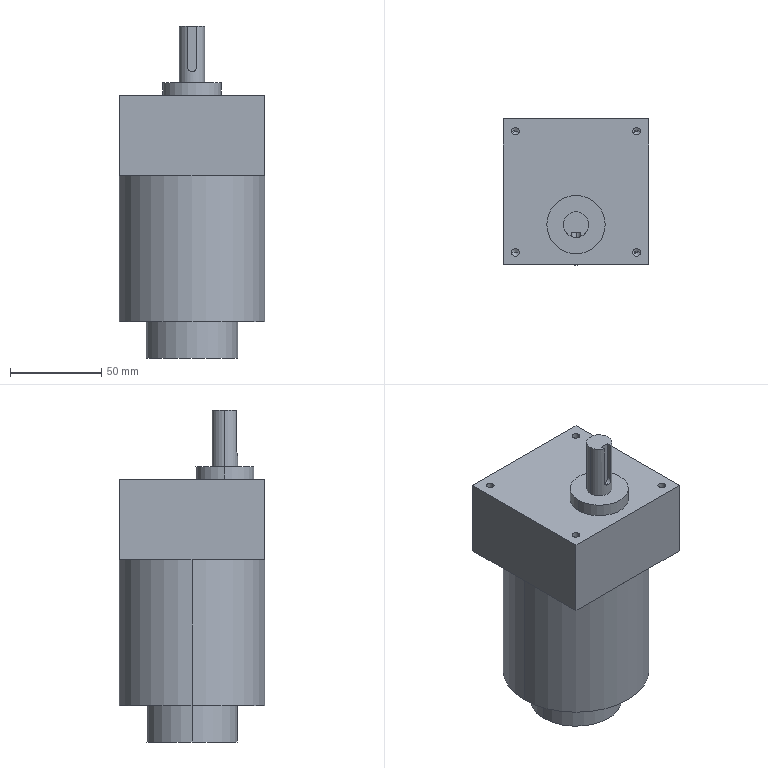Part | STEP file | Cut-off geared motor | 1 solid | 42 faces | box 80 x 80 x 182 mm | volume 732361 mm3 | cylinder 18 | plane 16 | cone 8 | commonest cylinder face diameters 4.2 x8 5 x2 14 x2 32 x2 50 x2 80 x2
STEP:
#1=CARTESIAN_POINT('',(31.134,-33.234,31.6));
#2=VERTEX_POINT('',#1);
#3=CARTESIAN_POINT('',(35.334,-33.234,31.6));
#4=VERTEX_POINT('',#3);
#5=CARTESIAN_POINT('',(33.234,-33.234,31.6));
#6=DIRECTION('',(0.,0.,1.));
#7=DIRECTION('',(1.,0.,0.));
#8=AXIS2_PLACEMENT_3D('',#5,#6,#7);
#9=CIRCLE('',#8,2.1);
#10=EDGE_CURVE('',#2,#4,#9,.T.);
#11=ORIENTED_EDGE('',*,*,#10,.F.);
#12=CARTESIAN_POINT('',(31.134,-33.234,44.));
#13=VERTEX_POINT('',#12);
#14=CARTESIAN_POINT('',(31.134,-33.234,44.));
#15=DIRECTION('',(0.,0.,1.));
#16=VECTOR('',#15,1000.);
#17=LINE('',#14,#16);
#18=EDGE_CURVE('',#2,#13,#17,.T.);
#19=ORIENTED_EDGE('',*,*,#18,.T.);
#20=CARTESIAN_POINT('',(35.334,-33.234,44.));
#21=VERTEX_POINT('',#20);
#22=CARTESIAN_POINT('',(33.234,-33.234,44.));
#23=DIRECTION('',(0.,0.,1.));
#24=DIRECTION('',(1.,0.,0.));
#25=AXIS2_PLACEMENT_3D('',#22,#23,#24);
#26=CIRCLE('',#25,2.1);
#27=EDGE_CURVE('',#13,#21,#26,.T.);
#28=ORIENTED_EDGE('',*,*,#27,.T.);
#29=CARTESIAN_POINT('',(35.334,-33.234,44.));
#30=DIRECTION('',(0.,0.,1.));
#31=VECTOR('',#30,1000.);
#32=LINE('',#29,#31);
#33=EDGE_CURVE('',#4,#21,#32,.T.);
#34=ORIENTED_EDGE('',*,*,#33,.F.);
#35=EDGE_LOOP('',(#11,#19,#28,#34));
#36=FACE_OUTER_BOUND('',#35,.T.);
#37=CARTESIAN_POINT('',(33.234,-33.234,44.));
#38=DIRECTION('',(0.,0.,1.));
#39=DIRECTION('',(1.,0.,0.));
#40=AXIS2_PLACEMENT_3D('',#37,#38,#39);
#41=CYLINDRICAL_SURFACE('',#40,2.1);
#42=ADVANCED_FACE('',(#36),#41,.F.);
#43=CARTESIAN_POINT('',(33.234,-33.234,30.338));
#44=VERTEX_POINT('',#43);
#45=CARTESIAN_POINT('',(35.334,-33.234,31.6));
#46=DIRECTION('',(0.8572,0.,0.515));
#47=VECTOR('',#46,1000.);
#48=LINE('',#45,#47);
#49=EDGE_CURVE('',#44,#4,#48,.T.);
#50=ORIENTED_EDGE('',*,*,#49,.F.);
#51=CARTESIAN_POINT('',(31.134,-33.234,31.6));
#52=DIRECTION('',(-0.8572,0.,0.515));
#53=VECTOR('',#52,1000.);
#54=LINE('',#51,#53);
#55=EDGE_CURVE('',#44,#2,#54,.T.);
#56=ORIENTED_EDGE('',*,*,#55,.T.);
#57=ORIENTED_EDGE('',*,*,#10,.T.);
#58=EDGE_LOOP('',(#50,#56,#57));
#59=FACE_OUTER_BOUND('',#58,.T.);
#60=CARTESIAN_POINT('',(33.234,-33.234,31.6));
#61=DIRECTION('',(0.,0.,1.));
#62=DIRECTION('',(1.,0.,0.));
#63=AXIS2_PLACEMENT_3D('',#60,#61,#62);
#64=CONICAL_SURFACE('',#63,2.1,1.03);
#65=ADVANCED_FACE('',(#59),#64,.F.);
#66=CARTESIAN_POINT('',(-35.334,-33.234,31.6));
#67=VERTEX_POINT('',#66);
#68=CARTESIAN_POINT('',(-31.134,-33.234,31.6));
#69=VERTEX_POINT('',#68);
#70=CARTESIAN_POINT('',(-33.234,-33.234,31.6));
#71=DIRECTION('',(0.,0.,1.));
#72=DIRECTION('',(1.,0.,0.));
#73=AXIS2_PLACEMENT_3D('',#70,#71,#72);
#74=CIRCLE('',#73,2.1);
#75=EDGE_CURVE('',#67,#69,#74,.T.);
#76=ORIENTED_EDGE('',*,*,#75,.F.);
#77=CARTESIAN_POINT('',(-35.334,-33.234,44.));
#78=VERTEX_POINT('',#77);
#79=CARTESIAN_POINT('',(-35.334,-33.234,44.));
#80=DIRECTION('',(0.,0.,1.));
#81=VECTOR('',#80,1000.);
#82=LINE('',#79,#81);
#83=EDGE_CURVE('',#67,#78,#82,.T.);
#84=ORIENTED_EDGE('',*,*,#83,.T.);
#85=CARTESIAN_POINT('',(-31.134,-33.234,44.));
#86=VERTEX_POINT('',#85);
#87=CARTESIAN_POINT('',(-33.234,-33.234,44.));
#88=DIRECTION('',(0.,0.,1.));
#89=DIRECTION('',(1.,0.,0.));
#90=AXIS2_PLACEMENT_3D('',#87,#88,#89);
#91=CIRCLE('',#90,2.1);
#92=EDGE_CURVE('',#78,#86,#91,.T.);
#93=ORIENTED_EDGE('',*,*,#92,.T.);
#94=CARTESIAN_POINT('',(-31.134,-33.234,44.));
#95=DIRECTION('',(0.,0.,1.));
#96=VECTOR('',#95,1000.);
#97=LINE('',#94,#96);
#98=EDGE_CURVE('',#69,#86,#97,.T.);
#99=ORIENTED_EDGE('',*,*,#98,.F.);
#100=EDGE_LOOP('',(#76,#84,#93,#99));
#101=FACE_OUTER_BOUND('',#100,.T.);
#102=CARTESIAN_POINT('',(-33.234,-33.234,44.));
#103=DIRECTION('',(0.,0.,1.));
#104=DIRECTION('',(1.,0.,0.));
#105=AXIS2_PLACEMENT_3D('',#102,#103,#104);
#106=CYLINDRICAL_SURFACE('',#105,2.1);
#107=ADVANCED_FACE('',(#101),#106,.F.);
#108=CARTESIAN_POINT('',(-33.234,-33.234,30.338));
#109=VERTEX_POINT('',#108);
#110=CARTESIAN_POINT('',(-31.134,-33.234,31.6));
#111=DIRECTION('',(0.8572,0.,0.515));
#112=VECTOR('',#111,1000.);
#113=LINE('',#110,#112);
#114=EDGE_CURVE('',#109,#69,#113,.T.);
#115=ORIENTED_EDGE('',*,*,#114,.F.);
#116=CARTESIAN_POINT('',(-35.334,-33.234,31.6));
#117=DIRECTION('',(-0.8572,0.,0.515));
#118=VECTOR('',#117,1000.);
#119=LINE('',#116,#118);
#120=EDGE_CURVE('',#109,#67,#119,.T.);
#121=ORIENTED_EDGE('',*,*,#120,.T.);
#122=ORIENTED_EDGE('',*,*,#75,.T.);
#123=EDGE_LOOP('',(#115,#121,#122));
#124=FACE_OUTER_BOUND('',#123,.T.);
#125=CARTESIAN_POINT('',(-33.234,-33.234,31.6));
#126=DIRECTION('',(0.,0.,1.));
#127=DIRECTION('',(1.,0.,0.));
#128=AXIS2_PLACEMENT_3D('',#125,#126,#127);
#129=CONICAL_SURFACE('',#128,2.1,1.03);
#130=ADVANCED_FACE('',(#124),#129,.F.);
#131=CARTESIAN_POINT('',(-35.334,33.234,31.6));
#132=VERTEX_POINT('',#131);
#133=CARTESIAN_POINT('',(-31.134,33.234,31.6));
#134=VERTEX_POINT('',#133);
#135=CARTESIAN_POINT('',(-33.234,33.234,31.6));
#136=DIRECTION('',(0.,0.,1.));
#137=DIRECTION('',(1.,0.,0.));
#138=AXIS2_PLACEMENT_3D('',#135,#136,#137);
#139=CIRCLE('',#138,2.1);
#140=EDGE_CURVE('',#132,#134,#139,.T.);
#141=ORIENTED_EDGE('',*,*,#140,.F.);
#142=CARTESIAN_POINT('',(-35.334,33.234,44.));
#143=VERTEX_POINT('',#142);
#144=CARTESIAN_POINT('',(-35.334,33.234,44.));
#145=DIRECTION('',(0.,0.,1.));
#146=VECTOR('',#145,1000.);
#147=LINE('',#144,#146);
#148=EDGE_CURVE('',#132,#143,#147,.T.);
#149=ORIENTED_EDGE('',*,*,#148,.T.);
#150=CARTESIAN_POINT('',(-31.134,33.234,44.));
#151=VERTEX_POINT('',#150);
#152=CARTESIAN_POINT('',(-33.234,33.234,44.));
#153=DIRECTION('',(0.,0.,1.));
#154=DIRECTION('',(1.,0.,0.));
#155=AXIS2_PLACEMENT_3D('',#152,#153,#154);
#156=CIRCLE('',#155,2.1);
#157=EDGE_CURVE('',#143,#151,#156,.T.);
#158=ORIENTED_EDGE('',*,*,#157,.T.);
#159=CARTESIAN_POINT('',(-31.134,33.234,44.));
#160=DIRECTION('',(0.,0.,1.));
#161=VECTOR('',#160,1000.);
#162=LINE('',#159,#161);
#163=EDGE_CURVE('',#134,#151,#162,.T.);
#164=ORIENTED_EDGE('',*,*,#163,.F.);
#165=EDGE_LOOP('',(#141,#149,#158,#164));
#166=FACE_OUTER_BOUND('',#165,.T.);
#167=CARTESIAN_POINT('',(-33.234,33.234,44.));
#168=DIRECTION('',(0.,0.,1.));
#169=DIRECTION('',(1.,0.,0.));
#170=AXIS2_PLACEMENT_3D('',#167,#168,#169);
#171=CYLINDRICAL_SURFACE('',#170,2.1);
#172=ADVANCED_FACE('',(#166),#171,.F.);
#173=CARTESIAN_POINT('',(-33.234,33.234,30.338));
#174=VERTEX_POINT('',#173);
#175=CARTESIAN_POINT('',(-31.134,33.234,31.6));
#176=DIRECTION('',(0.8572,0.,0.515));
#177=VECTOR('',#176,1000.);
#178=LINE('',#175,#177);
#179=EDGE_CURVE('',#174,#134,#178,.T.);
#180=ORIENTED_EDGE('',*,*,#179,.F.);
#181=CARTESIAN_POINT('',(-35.334,33.234,31.6));
#182=DIRECTION('',(-0.8572,0.,0.515));
#183=VECTOR('',#182,1000.);
#184=LINE('',#181,#183);
#185=EDGE_CURVE('',#174,#132,#184,.T.);
#186=ORIENTED_EDGE('',*,*,#185,.T.);
#187=ORIENTED_EDGE('',*,*,#140,.T.);
#188=EDGE_LOOP('',(#180,#186,#187));
#189=FACE_OUTER_BOUND('',#188,.T.);
#190=CARTESIAN_POINT('',(-33.234,33.234,31.6));
#191=DIRECTION('',(0.,0.,1.));
#192=DIRECTION('',(1.,0.,0.));
#193=AXIS2_PLACEMENT_3D('',#190,#191,#192);
#194=CONICAL_SURFACE('',#193,2.1,1.03);
#195=ADVANCED_FACE('',(#189),#194,.F.);
#196=CARTESIAN_POINT('',(31.134,33.234,31.6));
#197=VERTEX_POINT('',#196);
#198=CARTESIAN_POINT('',(35.334,33.234,31.6));
#199=VERTEX_POINT('',#198);
#200=CARTESIAN_POINT('',(33.234,33.234,31.6));
#201=DIRECTION('',(0.,0.,1.));
#202=DIRECTION('',(1.,0.,0.));
#203=AXIS2_PLACEMENT_3D('',#200,#201,#202);
#204=CIRCLE('',#203,2.1);
#205=EDGE_CURVE('',#197,#199,#204,.T.);
#206=ORIENTED_EDGE('',*,*,#205,.F.);
#207=CARTESIAN_POINT('',(31.134,33.234,44.));
#208=VERTEX_POINT('',#207);
#209=CARTESIAN_POINT('',(31.134,33.234,44.));
#210=DIRECTION('',(0.,0.,1.));
#211=VECTOR('',#210,1000.);
#212=LINE('',#209,#211);
#213=EDGE_CURVE('',#197,#208,#212,.T.);
#214=ORIENTED_EDGE('',*,*,#213,.T.);
#215=CARTESIAN_POINT('',(35.334,33.234,44.));
#216=VERTEX_POINT('',#215);
#217=CARTESIAN_POINT('',(33.234,33.234,44.));
#218=DIRECTION('',(0.,0.,1.));
#219=DIRECTION('',(1.,0.,0.));
#220=AXIS2_PLACEMENT_3D('',#217,#218,#219);
#221=CIRCLE('',#220,2.1);
#222=EDGE_CURVE('',#208,#216,#221,.T.);
#223=ORIENTED_EDGE('',*,*,#222,.T.);
#224=CARTESIAN_POINT('',(35.334,33.234,44.));
#225=DIRECTION('',(0.,0.,1.));
#226=VECTOR('',#225,1000.);
#227=LINE('',#224,#226);
#228=EDGE_CURVE('',#199,#216,#227,.T.);
#229=ORIENTED_EDGE('',*,*,#228,.F.);
#230=EDGE_LOOP('',(#206,#214,#223,#229));
#231=FACE_OUTER_BOUND('',#230,.T.);
#232=CARTESIAN_POINT('',(33.234,33.234,44.));
#233=DIRECTION('',(0.,0.,1.));
#234=DIRECTION('',(1.,0.,0.));
#235=AXIS2_PLACEMENT_3D('',#232,#233,#234);
#236=CYLINDRICAL_SURFACE('',#235,2.1);
#237=ADVANCED_FACE('',(#231),#236,.F.);
#238=CARTESIAN_POINT('',(33.234,33.234,30.338));
#239=VERTEX_POINT('',#238);
#240=CARTESIAN_POINT('',(35.334,33.234,31.6));
#241=DIRECTION('',(0.8572,0.,0.515));
#242=VECTOR('',#241,1000.);
#243=LINE('',#240,#242);
#244=EDGE_CURVE('',#239,#199,#243,.T.);
#245=ORIENTED_EDGE('',*,*,#244,.F.);
#246=CARTESIAN_POINT('',(31.134,33.234,31.6));
#247=DIRECTION('',(-0.8572,0.,0.515));
#248=VECTOR('',#247,1000.);
#249=LINE('',#246,#248);
#250=EDGE_CURVE('',#239,#197,#249,.T.);
#251=ORIENTED_EDGE('',*,*,#250,.T.);
#252=ORIENTED_EDGE('',*,*,#205,.T.);
#253=EDGE_LOOP('',(#245,#251,#252));
#254=FACE_OUTER_BOUND('',#253,.T.);
#255=CARTESIAN_POINT('',(33.234,33.234,31.6));
#256=DIRECTION('',(0.,0.,1.));
#257=DIRECTION('',(1.,0.,0.));
#258=AXIS2_PLACEMENT_3D('',#255,#256,#257);
#259=CONICAL_SURFACE('',#258,2.1,1.03);
#260=ADVANCED_FACE('',(#254),#259,.F.);
#261=CARTESIAN_POINT('',(7.,-18.,82.));
#262=VERTEX_POINT('',#261);
#263=CARTESIAN_POINT('',(-7.,-18.,82.));
#264=VERTEX_POINT('',#263);
#265=CARTESIAN_POINT('',(0.,-18.,82.));
#266=DIRECTION('',(0.,0.,1.));
#267=DIRECTION('',(1.,0.,0.));
#268=AXIS2_PLACEMENT_3D('',#265,#266,#267);
#269=CIRCLE('',#268,7.);
#270=EDGE_CURVE('',#262,#264,#269,.T.);
#271=ORIENTED_EDGE('',*,*,#270,.F.);
#272=CARTESIAN_POINT('',(7.,-18.,51.));
#273=VERTEX_POINT('',#272);
#274=CARTESIAN_POINT('',(7.,-18.,82.));
#275=DIRECTION('',(0.,0.,-1.));
#276=VECTOR('',#275,1000.);
#277=LINE('',#274,#276);
#278=EDGE_CURVE('',#262,#273,#277,.T.);
#279=ORIENTED_EDGE('',*,*,#278,.T.);
#280=CARTESIAN_POINT('',(-7.,-18.,51.));
#281=VERTEX_POINT('',#280);
#282=CARTESIAN_POINT('',(0.,-18.,51.));
#283=DIRECTION('',(0.,0.,1.));
#284=DIRECTION('',(1.,0.,0.));
#285=AXIS2_PLACEMENT_3D('',#282,#283,#284);
#286=CIRCLE('',#285,7.);
#287=EDGE_CURVE('',#273,#281,#286,.T.);
#288=ORIENTED_EDGE('',*,*,#287,.T.);
#289=CARTESIAN_POINT('',(-7.,-18.,82.));
#290=DIRECTION('',(0.,0.,-1.));
#291=VECTOR('',#290,1000.);
#292=LINE('',#289,#291);
#293=EDGE_CURVE('',#264,#281,#292,.T.);
#294=ORIENTED_EDGE('',*,*,#293,.F.);
#295=EDGE_LOOP('',(#271,#279,#288,#294));
#296=FACE_OUTER_BOUND('',#295,.T.);
#297=CARTESIAN_POINT('',(0.,-18.,82.));
#298=DIRECTION('',(0.,0.,-1.));
#299=DIRECTION('',(-1.,0.,0.));
#300=AXIS2_PLACEMENT_3D('',#297,#298,#299);
#301=CYLINDRICAL_SURFACE('',#300,7.);
#302=ADVANCED_FACE('',(#296),#301,.T.);
#303=CARTESIAN_POINT('',(16.,-18.,51.));
#304=VERTEX_POINT('',#303);
#305=CARTESIAN_POINT('',(-16.,-18.,51.));
#306=VERTEX_POINT('',#305);
#307=CARTESIAN_POINT('',(0.,-18.,51.));
#308=DIRECTION('',(0.,0.,1.));
#309=DIRECTION('',(1.,0.,0.));
#310=AXIS2_PLACEMENT_3D('',#307,#308,#309);
#311=CIRCLE('',#310,16.);
#312=EDGE_CURVE('',#304,#306,#311,.T.);
#313=ORIENTED_EDGE('',*,*,#312,.F.);
#314=CARTESIAN_POINT('',(16.,-18.,44.));
#315=VERTEX_POINT('',#314);
#316=CARTESIAN_POINT('',(16.,-18.,51.));
#317=DIRECTION('',(0.,0.,-1.));
#318=VECTOR('',#317,1000.);
#319=LINE('',#316,#318);
#320=EDGE_CURVE('',#304,#315,#319,.T.);
#321=ORIENTED_EDGE('',*,*,#320,.T.);
#322=CARTESIAN_POINT('',(-16.,-18.,44.));
#323=VERTEX_POINT('',#322);
#324=CARTESIAN_POINT('',(0.,-18.,44.));
#325=DIRECTION('',(0.,0.,1.));
#326=DIRECTION('',(1.,0.,0.));
#327=AXIS2_PLACEMENT_3D('',#324,#325,#326);
#328=CIRCLE('',#327,16.);
#329=EDGE_CURVE('',#315,#323,#328,.T.);
#330=ORIENTED_EDGE('',*,*,#329,.T.);
#331=CARTESIAN_POINT('',(-16.,-18.,51.));
#332=DIRECTION('',(0.,0.,-1.));
#333=VECTOR('',#332,1000.);
#334=LINE('',#331,#333);
#335=EDGE_CURVE('',#306,#323,#334,.T.);
#336=ORIENTED_EDGE('',*,*,#335,.F.);
#337=EDGE_LOOP('',(#313,#321,#330,#336));
#338=FACE_OUTER_BOUND('',#337,.T.);
#339=CARTESIAN_POINT('',(0.,-18.,51.));
#340=DIRECTION('',(0.,0.,-1.));
#341=DIRECTION('',(-1.,0.,0.));
#342=AXIS2_PLACEMENT_3D('',#339,#340,#341);
#343=CYLINDRICAL_SURFACE('',#342,16.);
#344=ADVANCED_FACE('',(#338),#343,.T.);
#345=CARTESIAN_POINT('',(-25.,0.,-100.));
#346=VERTEX_POINT('',#345);
#347=CARTESIAN_POINT('',(25.,0.,-100.));
#348=VERTEX_POINT('',#347);
#349=CARTESIAN_POINT('',(0.,0.,-100.));
#350=DIRECTION('',(0.,0.,-1.));
#351=DIRECTION('',(-1.,0.,0.));
#352=AXIS2_PLACEMENT_3D('',#349,#350,#351);
#353=CIRCLE('',#352,25.);
#354=EDGE_CURVE('',#346,#348,#353,.T.);
#355=ORIENTED_EDGE('',*,*,#354,.F.);
#356=CARTESIAN_POINT('',(-25.,0.,-80.));
#357=VERTEX_POINT('',#356);
#358=CARTESIAN_POINT('',(-25.,0.,-100.));
#359=DIRECTION('',(0.,0.,1.));
#360=VECTOR('',#359,1000.);
#361=LINE('',#358,#360);
#362=EDGE_CURVE('',#346,#357,#361,.T.);
#363=ORIENTED_EDGE('',*,*,#362,.T.);
#364=CARTESIAN_POINT('',(25.,0.,-80.));
#365=VERTEX_POINT('',#364);
#366=CARTESIAN_POINT('',(0.,0.,-80.));
#367=DIRECTION('',(0.,0.,-1.));
#368=DIRECTION('',(-1.,0.,0.));
#369=AXIS2_PLACEMENT_3D('',#366,#367,#368);
#370=CIRCLE('',#369,25.);
#371=EDGE_CURVE('',#357,#365,#370,.T.);
#372=ORIENTED_EDGE('',*,*,#371,.T.);
#373=CARTESIAN_POINT('',(25.,0.,-100.));
#374=DIRECTION('',(0.,0.,1.));
#375=VECTOR('',#374,1000.);
#376=LINE('',#373,#375);
#377=EDGE_CURVE('',#348,#365,#376,.T.);
#378=ORIENTED_EDGE('',*,*,#377,.F.);
#379=EDGE_LOOP('',(#355,#363,#372,#378));
#380=FACE_OUTER_BOUND('',#379,.T.);
#381=CARTESIAN_POINT('',(0.,0.,-100.));
#382=DIRECTION('',(0.,0.,1.));
#383=DIRECTION('',(1.,0.,0.));
#384=AXIS2_PLACEMENT_3D('',#381,#382,#383);
#385=CYLINDRICAL_SURFACE('',#384,25.);
#386=ADVANCED_FACE('',(#380),#385,.T.);
#387=CARTESIAN_POINT('',(-40.,0.,-80.));
#388=VERTEX_POINT('',#387);
#389=CARTESIAN_POINT('',(40.,0.,-80.));
#390=VERTEX_POINT('',#389);
#391=CARTESIAN_POINT('',(0.,0.,-80.));
#392=DIRECTION('',(0.,0.,-1.));
#393=DIRECTION('',(-1.,0.,0.));
#394=AXIS2_PLACEMENT_3D('',#391,#392,#393);
#395=CIRCLE('',#394,40.);
#396=EDGE_CURVE('',#388,#390,#395,.T.);
#397=ORIENTED_EDGE('',*,*,#396,.F.);
#398=CARTESIAN_POINT('',(-40.,0.,0.));
#399=VERTEX_POINT('',#398);
#400=CARTESIAN_POINT('',(-40.,0.,-80.));
#401=DIRECTION('',(0.,0.,1.));
#402=VECTOR('',#401,1000.);
#403=LINE('',#400,#402);
#404=EDGE_CURVE('',#388,#399,#403,.T.);
#405=ORIENTED_EDGE('',*,*,#404,.T.);
#406=CARTESIAN_POINT('',(0.,40.,0.));
#407=VERTEX_POINT('',#406);
#408=CARTESIAN_POINT('',(0.,0.,0.));
#409=DIRECTION('',(0.,0.,-1.));
#410=DIRECTION('',(-1.,0.,0.));
#411=AXIS2_PLACEMENT_3D('',#408,#409,#410);
#412=CIRCLE('',#411,40.);
#413=EDGE_CURVE('',#399,#407,#412,.T.);
#414=ORIENTED_EDGE('',*,*,#413,.T.);
#415=CARTESIAN_POINT('',(40.,0.,0.));
#416=VERTEX_POINT('',#415);
#417=CARTESIAN_POINT('',(0.,0.,0.));
#418=DIRECTION('',(0.,0.,-1.));
#419=DIRECTION('',(-1.,0.,0.));
#420=AXIS2_PLACEMENT_3D('',#417,#418,#419);
#421=CIRCLE('',#420,40.);
#422=EDGE_CURVE('',#407,#416,#421,.T.);
#423=ORIENTED_EDGE('',*,*,#422,.T.);
#424=CARTESIAN_POINT('',(40.,0.,-80.));
#425=DIRECTION('',(0.,0.,1.));
#426=VECTOR('',#425,1000.);
#427=LINE('',#424,#426);
#428=EDGE_CURVE('',#390,#416,#427,.T.);
#429=ORIENTED_EDGE('',*,*,#428,.F.);
#430=EDGE_LOOP('',(#397,#405,#414,#423,#429));
#431=FACE_OUTER_BOUND('',#430,.T.);
#432=CARTESIAN_POINT('',(0.,0.,-80.));
#433=DIRECTION('',(0.,0.,1.));
#434=DIRECTION('',(1.,0.,0.));
#435=AXIS2_PLACEMENT_3D('',#432,#433,#434);
#436=CYLINDRICAL_SURFACE('',#435,40.);
#437=ADVANCED_FACE('',(#431),#436,.T.);
#438=ORIENTED_EDGE('',*,*,#413,.F.);
#439=CARTESIAN_POINT('',(-40.,40.,0.));
#440=VERTEX_POINT('',#439);
#441=CARTESIAN_POINT('',(-40.,40.,0.));
#442=DIRECTION('',(0.,-1.,0.));
#443=VECTOR('',#442,1000.);
#444=LINE('',#441,#443);
#445=EDGE_CURVE('',#440,#399,#444,.T.);
#446=ORIENTED_EDGE('',*,*,#445,.F.);
#447=CARTESIAN_POINT('',(-40.,40.,0.));
#448=DIRECTION('',(-1.,0.,0.));
#449=VECTOR('',#448,1000.);
#450=LINE('',#447,#449);
#451=EDGE_CURVE('',#407,#440,#450,.T.);
#452=ORIENTED_EDGE('',*,*,#451,.F.);
#453=EDGE_LOOP('',(#438,#446,#452));
#454=FACE_OUTER_BOUND('',#453,.T.);
#455=CARTESIAN_POINT('',(0.,0.,0.));
#456=DIRECTION('',(0.,0.,1.));
#457=DIRECTION('',(1.,0.,0.));
#458=AXIS2_PLACEMENT_3D('',#455,#456,#457);
#459=PLANE('',#458);
#460=ADVANCED_FACE('',(#454),#459,.F.);
#461=ORIENTED_EDGE('',*,*,#422,.F.);
#462=CARTESIAN_POINT('',(40.,40.,0.));
#463=VERTEX_POINT('',#462);
#464=CARTESIAN_POINT('',(-40.,40.,0.));
#465=DIRECTION('',(-1.,0.,0.));
#466=VECTOR('',#465,1000.);
#467=LINE('',#464,#466);
#468=EDGE_CURVE('',#463,#407,#467,.T.);
#469=ORIENTED_EDGE('',*,*,#468,.F.);
#470=CARTESIAN_POINT('',(40.,40.,0.));
#471=DIRECTION('',(0.,1.,0.));
#472=VECTOR('',#471,1000.);
#473=LINE('',#470,#472);
#474=EDGE_CURVE('',#416,#463,#473,.T.);
#475=ORIENTED_EDGE('',*,*,#474,.F.);
#476=EDGE_LOOP('',(#461,#469,#475));
#477=FACE_OUTER_BOUND('',#476,.T.);
#478=CARTESIAN_POINT('',(0.,0.,0.));
#479=DIRECTION('',(0.,0.,1.));
#480=DIRECTION('',(1.,0.,0.));
#481=AXIS2_PLACEMENT_3D('',#478,#479,#480);
#482=PLANE('',#481);
#483=ADVANCED_FACE('',(#477),#482,.F.);
#484=CARTESIAN_POINT('',(0.,-40.,0.));
#485=VERTEX_POINT('',#484);
#486=CARTESIAN_POINT('',(0.,0.,0.));
#487=DIRECTION('',(0.,0.,-1.));
#488=DIRECTION('',(-1.,0.,0.));
#489=AXIS2_PLACEMENT_3D('',#486,#487,#488);
#490=CIRCLE('',#489,40.);
#491=EDGE_CURVE('',#416,#485,#490,.T.);
#492=ORIENTED_EDGE('',*,*,#491,.F.);
#493=CARTESIAN_POINT('',(40.,-40.,0.));
#494=VERTEX_POINT('',#493);
#495=CARTESIAN_POINT('',(40.,40.,0.));
#496=DIRECTION('',(0.,1.,0.));
#497=VECTOR('',#496,1000.);
#498=LINE('',#495,#497);
#499=EDGE_CURVE('',#494,#416,#498,.T.);
#500=ORIENTED_EDGE('',*,*,#499,.F.);
#501=CARTESIAN_POINT('',(-40.,-40.,0.));
#502=DIRECTION('',(1.,0.,0.));
#503=VECTOR('',#502,1000.);
#504=LINE('',#501,#503);
#505=EDGE_CURVE('',#485,#494,#504,.T.);
#506=ORIENTED_EDGE('',*,*,#505,.F.);
#507=EDGE_LOOP('',(#492,#500,#506));
#508=FACE_OUTER_BOUND('',#507,.T.);
#509=CARTESIAN_POINT('',(0.,0.,0.));
#510=DIRECTION('',(0.,0.,1.));
#511=DIRECTION('',(1.,0.,0.));
#512=AXIS2_PLACEMENT_3D('',#509,#510,#511);
#513=PLANE('',#512);
#514=ADVANCED_FACE('',(#508),#513,.F.);
#515=ORIENTED_EDGE('',*,*,#499,.T.);
#516=ORIENTED_EDGE('',*,*,#474,.T.);
#517=CARTESIAN_POINT('',(40.,40.,44.));
#518=VERTEX_POINT('',#517);
#519=CARTESIAN_POINT('',(40.,40.,44.));
#520=DIRECTION('',(0.,0.,-1.));
#521=VECTOR('',#520,1000.);
#522=LINE('',#519,#521);
#523=EDGE_CURVE('',#518,#463,#522,.T.);
#524=ORIENTED_EDGE('',*,*,#523,.F.);
#525=CARTESIAN_POINT('',(40.,-40.,44.));
#526=VERTEX_POINT('',#525);
#527=CARTESIAN_POINT('',(40.,40.,44.));
#528=DIRECTION('',(0.,1.,0.));
#529=VECTOR('',#528,1000.);
#530=LINE('',#527,#529);
#531=EDGE_CURVE('',#526,#518,#530,.T.);
#532=ORIENTED_EDGE('',*,*,#531,.F.);
#533=CARTESIAN_POINT('',(40.,-40.,44.));
#534=DIRECTION('',(0.,0.,-1.));
#535=VECTOR('',#534,1000.);
#536=LINE('',#533,#535);
#537=EDGE_CURVE('',#526,#494,#536,.T.);
#538=ORIENTED_EDGE('',*,*,#537,.T.);
#539=EDGE_LOOP('',(#515,#516,#524,#532,#538));
#540=FACE_OUTER_BOUND('',#539,.T.);
#541=CARTESIAN_POINT('',(40.,40.,44.));
#542=DIRECTION('',(-1.,0.,0.));
#543=DIRECTION('',(0.,0.,1.));
#544=AXIS2_PLACEMENT_3D('',#541,#542,#543);
#545=PLANE('',#544);
#546=ADVANCED_FACE('',(#540),#545,.F.);
#547=ORIENTED_EDGE('',*,*,#468,.T.);
#548=ORIENTED_EDGE('',*,*,#451,.T.);
#549=CARTESIAN_POINT('',(-40.,40.,44.));
#550=VERTEX_POINT('',#549);
#551=CARTESIAN_POINT('',(-40.,40.,44.));
#552=DIRECTION('',(0.,0.,-1.));
#553=VECTOR('',#552,1000.);
#554=LINE('',#551,#553);
#555=EDGE_CURVE('',#550,#440,#554,.T.);
#556=ORIENTED_EDGE('',*,*,#555,.F.);
#557=CARTESIAN_POINT('',(-40.,40.,44.));
#558=DIRECTION('',(-1.,0.,0.));
#559=VECTOR('',#558,1000.);
#560=LINE('',#557,#559);
#561=EDGE_CURVE('',#518,#550,#560,.T.);
#562=ORIENTED_EDGE('',*,*,#561,.F.);
#563=ORIENTED_EDGE('',*,*,#523,.T.);
#564=EDGE_LOOP('',(#547,#548,#556,#562,#563));
#565=FACE_OUTER_BOUND('',#564,.T.);
#566=CARTESIAN_POINT('',(-40.,40.,44.));
#567=DIRECTION('',(0.,-1.,0.));
#568=DIRECTION('',(0.,0.,-1.));
#569=AXIS2_PLACEMENT_3D('',#566,#567,#568);
#570=PLANE('',#569);
#571=ADVANCED_FACE('',(#565),#570,.F.);
#572=ORIENTED_EDGE('',*,*,#445,.T.);
#573=CARTESIAN_POINT('',(-40.,-40.,0.));
#574=VERTEX_POINT('',#573);
#575=CARTESIAN_POINT('',(-40.,40.,0.));
#576=DIRECTION('',(0.,-1.,0.));
#577=VECTOR('',#576,1000.);
#578=LINE('',#575,#577);
#579=EDGE_CURVE('',#399,#574,#578,.T.);
#580=ORIENTED_EDGE('',*,*,#579,.T.);
#581=CARTESIAN_POINT('',(-40.,-40.,44.));
#582=VERTEX_POINT('',#581);
#583=CARTESIAN_POINT('',(-40.,-40.,44.));
#584=DIRECTION('',(0.,0.,-1.));
#585=VECTOR('',#584,1000.);
#586=LINE('',#583,#585);
#587=EDGE_CURVE('',#582,#574,#586,.T.);
#588=ORIENTED_EDGE('',*,*,#587,.F.);
#589=CARTESIAN_POINT('',(-40.,40.,44.));
#590=DIRECTION('',(0.,-1.,0.));
#591=VECTOR('',#590,1000.);
#592=LINE('',#589,#591);
#593=EDGE_CURVE('',#550,#582,#592,.T.);
#594=ORIENTED_EDGE('',*,*,#593,.F.);
#595=ORIENTED_EDGE('',*,*,#555,.T.);
#596=EDGE_LOOP('',(#572,#580,#588,#594,#595));
#597=FACE_OUTER_BOUND('',#596,.T.);
#598=CARTESIAN_POINT('',(-40.,40.,44.));
#599=DIRECTION('',(1.,0.,0.));
#600=DIRECTION('',(0.,0.,-1.));
#601=AXIS2_PLACEMENT_3D('',#598,#599,#600);
#602=PLANE('',#601);
#603=ADVANCED_FACE('',(#597),#602,.F.);
#604=CARTESIAN_POINT('',(-40.,-40.,0.));
#605=DIRECTION('',(1.,0.,0.));
#606=VECTOR('',#605,1000.);
#607=LINE('',#604,#606);
#608=EDGE_CURVE('',#574,#485,#607,.T.);
#609=ORIENTED_EDGE('',*,*,#608,.T.);
#610=ORIENTED_EDGE('',*,*,#505,.T.);
#611=ORIENTED_EDGE('',*,*,#537,.F.);
#612=CARTESIAN_POINT('',(-40.,-40.,44.));
#613=DIRECTION('',(1.,0.,0.));
#614=VECTOR('',#613,1000.);
#615=LINE('',#612,#614);
#616=EDGE_CURVE('',#582,#526,#615,.T.);
#617=ORIENTED_EDGE('',*,*,#616,.F.);
#618=ORIENTED_EDGE('',*,*,#587,.T.);
#619=EDGE_LOOP('',(#609,#610,#611,#617,#618));
#620=FACE_OUTER_BOUND('',#619,.T.);
#621=CARTESIAN_POINT('',(-40.,-40.,44.));
#622=DIRECTION('',(0.,1.,0.));
#623=DIRECTION('',(0.,0.,1.));
#624=AXIS2_PLACEMENT_3D('',#621,#622,#623);
#625=PLANE('',#624);
#626=ADVANCED_FACE('',(#620),#625,.F.);
#627=CARTESIAN_POINT('',(33.234,-33.234,44.));
#628=DIRECTION('',(0.,0.,1.));
#629=DIRECTION('',(1.,0.,0.));
#630=AXIS2_PLACEMENT_3D('',#627,#628,#629);
#631=CIRCLE('',#630,2.1);
#632=EDGE_CURVE('',#21,#13,#631,.T.);
#633=ORIENTED_EDGE('',*,*,#632,.F.);
#634=ORIENTED_EDGE('',*,*,#27,.F.);
#635=EDGE_LOOP('',(#633,#634));
#636=FACE_BOUND('',#635,.T.);
#637=CARTESIAN_POINT('',(-33.234,-33.234,44.));
#638=DIRECTION('',(0.,0.,1.));
#639=DIRECTION('',(1.,0.,0.));
#640=AXIS2_PLACEMENT_3D('',#637,#638,#639);
#641=CIRCLE('',#640,2.1);
#642=EDGE_CURVE('',#86,#78,#641,.T.);
#643=ORIENTED_EDGE('',*,*,#642,.F.);
#644=ORIENTED_EDGE('',*,*,#92,.F.);
#645=EDGE_LOOP('',(#643,#644));
#646=FACE_BOUND('',#645,.T.);
#647=CARTESIAN_POINT('',(-33.234,33.234,44.));
#648=DIRECTION('',(0.,0.,1.));
#649=DIRECTION('',(1.,0.,0.));
#650=AXIS2_PLACEMENT_3D('',#647,#648,#649);
#651=CIRCLE('',#650,2.1);
#652=EDGE_CURVE('',#151,#143,#651,.T.);
#653=ORIENTED_EDGE('',*,*,#652,.F.);
#654=ORIENTED_EDGE('',*,*,#157,.F.);
#655=EDGE_LOOP('',(#653,#654));
#656=FACE_BOUND('',#655,.T.);
#657=CARTESIAN_POINT('',(33.234,33.234,44.));
#658=DIRECTION('',(0.,0.,1.));
#659=DIRECTION('',(1.,0.,0.));
#660=AXIS2_PLACEMENT_3D('',#657,#658,#659);
#661=CIRCLE('',#660,2.1);
#662=EDGE_CURVE('',#216,#208,#661,.T.);
#663=ORIENTED_EDGE('',*,*,#662,.F.);
#664=ORIENTED_EDGE('',*,*,#222,.F.);
#665=EDGE_LOOP('',(#663,#664));
#666=FACE_BOUND('',#665,.T.);
#667=CARTESIAN_POINT('',(0.,-18.,44.));
#668=DIRECTION('',(0.,0.,1.));
#669=DIRECTION('',(1.,0.,0.));
#670=AXIS2_PLACEMENT_3D('',#667,#668,#669);
#671=CIRCLE('',#670,16.);
#672=EDGE_CURVE('',#323,#315,#671,.T.);
#673=ORIENTED_EDGE('',*,*,#672,.F.);
#674=ORIENTED_EDGE('',*,*,#329,.F.);
#675=EDGE_LOOP('',(#673,#674));
#676=FACE_BOUND('',#675,.T.);
#677=ORIENTED_EDGE('',*,*,#531,.T.);
#678=ORIENTED_EDGE('',*,*,#561,.T.);
#679=ORIENTED_EDGE('',*,*,#593,.T.);
#680=ORIENTED_EDGE('',*,*,#616,.T.);
#681=EDGE_LOOP('',(#677,#678,#679,#680));
#682=FACE_OUTER_BOUND('',#681,.T.);
#683=CARTESIAN_POINT('',(0.,0.,44.));
#684=DIRECTION('',(0.,0.,1.));
#685=DIRECTION('',(1.,0.,0.));
#686=AXIS2_PLACEMENT_3D('',#683,#684,#685);
#687=PLANE('',#686);
#688=ADVANCED_FACE('',(#636,#646,#656,#666,#676,#682),#687,.T.);
#689=CARTESIAN_POINT('',(0.,0.,0.));
#690=DIRECTION('',(0.,0.,-1.));
#691=DIRECTION('',(-1.,0.,0.));
#692=AXIS2_PLACEMENT_3D('',#689,#690,#691);
#693=CIRCLE('',#692,40.);
#694=EDGE_CURVE('',#485,#399,#693,.T.);
#695=ORIENTED_EDGE('',*,*,#694,.F.);
#696=ORIENTED_EDGE('',*,*,#608,.F.);
#697=ORIENTED_EDGE('',*,*,#579,.F.);
#698=EDGE_LOOP('',(#695,#696,#697));
#699=FACE_OUTER_BOUND('',#698,.T.);
#700=CARTESIAN_POINT('',(0.,0.,0.));
#701=DIRECTION('',(0.,0.,1.));
#702=DIRECTION('',(1.,0.,0.));
#703=AXIS2_PLACEMENT_3D('',#700,#701,#702);
#704=PLANE('',#703);
#705=ADVANCED_FACE('',(#699),#704,.F.);
#706=ORIENTED_EDGE('',*,*,#404,.F.);
#707=CARTESIAN_POINT('',(0.,0.,-80.));
#708=DIRECTION('',(0.,0.,-1.));
#709=DIRECTION('',(-1.,0.,0.));
#710=AXIS2_PLACEMENT_3D('',#707,#708,#709);
#711=CIRCLE('',#710,40.);
#712=EDGE_CURVE('',#390,#388,#711,.T.);
#713=ORIENTED_EDGE('',*,*,#712,.F.);
#714=ORIENTED_EDGE('',*,*,#428,.T.);
#715=ORIENTED_EDGE('',*,*,#491,.T.);
#716=ORIENTED_EDGE('',*,*,#694,.T.);
#717=EDGE_LOOP('',(#706,#713,#714,#715,#716));
#718=FACE_OUTER_BOUND('',#717,.T.);
#719=CARTESIAN_POINT('',(0.,0.,-80.));
#720=DIRECTION('',(0.,0.,1.));
#721=DIRECTION('',(1.,0.,0.));
#722=AXIS2_PLACEMENT_3D('',#719,#720,#721);
#723=CYLINDRICAL_SURFACE('',#722,40.);
#724=ADVANCED_FACE('',(#718),#723,.T.);
#725=CARTESIAN_POINT('',(0.,0.,-80.));
#726=DIRECTION('',(0.,0.,-1.));
#727=DIRECTION('',(-1.,0.,0.));
#728=AXIS2_PLACEMENT_3D('',#725,#726,#727);
#729=CIRCLE('',#728,25.);
#730=EDGE_CURVE('',#365,#357,#729,.T.);
#731=ORIENTED_EDGE('',*,*,#730,.F.);
#732=ORIENTED_EDGE('',*,*,#371,.F.);
#733=EDGE_LOOP('',(#731,#732));
#734=FACE_BOUND('',#733,.T.);
#735=ORIENTED_EDGE('',*,*,#712,.T.);
#736=ORIENTED_EDGE('',*,*,#396,.T.);
#737=EDGE_LOOP('',(#735,#736));
#738=FACE_OUTER_BOUND('',#737,.T.);
#739=CARTESIAN_POINT('',(0.,0.,-80.));
#740=DIRECTION('',(0.,0.,-1.));
#741=DIRECTION('',(-1.,0.,0.));
#742=AXIS2_PLACEMENT_3D('',#739,#740,#741);
#743=PLANE('',#742);
#744=ADVANCED_FACE('',(#734,#738),#743,.T.);
#745=ORIENTED_EDGE('',*,*,#362,.F.);
#746=CARTESIAN_POINT('',(0.,0.,-100.));
#747=DIRECTION('',(0.,0.,-1.));
#748=DIRECTION('',(-1.,0.,0.));
#749=AXIS2_PLACEMENT_3D('',#746,#747,#748);
#750=CIRCLE('',#749,25.);
#751=EDGE_CURVE('',#348,#346,#750,.T.);
#752=ORIENTED_EDGE('',*,*,#751,.F.);
#753=ORIENTED_EDGE('',*,*,#377,.T.);
#754=ORIENTED_EDGE('',*,*,#730,.T.);
#755=EDGE_LOOP('',(#745,#752,#753,#754));
#756=FACE_OUTER_BOUND('',#755,.T.);
#757=CARTESIAN_POINT('',(0.,0.,-100.));
#758=DIRECTION('',(0.,0.,1.));
#759=DIRECTION('',(1.,0.,0.));
#760=AXIS2_PLACEMENT_3D('',#757,#758,#759);
#761=CYLINDRICAL_SURFACE('',#760,25.);
#762=ADVANCED_FACE('',(#756),#761,.T.);
#763=ORIENTED_EDGE('',*,*,#751,.T.);
#764=ORIENTED_EDGE('',*,*,#354,.T.);
#765=EDGE_LOOP('',(#763,#764));
#766=FACE_OUTER_BOUND('',#765,.T.);
#767=CARTESIAN_POINT('',(0.,0.,-100.));
#768=DIRECTION('',(0.,0.,-1.));
#769=DIRECTION('',(-1.,0.,0.));
#770=AXIS2_PLACEMENT_3D('',#767,#768,#769);
#771=PLANE('',#770);
#772=ADVANCED_FACE('',(#766),#771,.T.);
#773=ORIENTED_EDGE('',*,*,#320,.F.);
#774=CARTESIAN_POINT('',(0.,-18.,51.));
#775=DIRECTION('',(0.,0.,1.));
#776=DIRECTION('',(1.,0.,0.));
#777=AXIS2_PLACEMENT_3D('',#774,#775,#776);
#778=CIRCLE('',#777,16.);
#779=EDGE_CURVE('',#306,#304,#778,.T.);
#780=ORIENTED_EDGE('',*,*,#779,.F.);
#781=ORIENTED_EDGE('',*,*,#335,.T.);
#782=ORIENTED_EDGE('',*,*,#672,.T.);
#783=EDGE_LOOP('',(#773,#780,#781,#782));
#784=FACE_OUTER_BOUND('',#783,.T.);
#785=CARTESIAN_POINT('',(0.,-18.,51.));
#786=DIRECTION('',(0.,0.,-1.));
#787=DIRECTION('',(-1.,0.,0.));
#788=AXIS2_PLACEMENT_3D('',#785,#786,#787);
#789=CYLINDRICAL_SURFACE('',#788,16.);
#790=ADVANCED_FACE('',(#784),#789,.T.);
#791=CARTESIAN_POINT('',(0.,-18.,51.));
#792=DIRECTION('',(0.,0.,1.));
#793=DIRECTION('',(1.,0.,0.));
#794=AXIS2_PLACEMENT_3D('',#791,#792,#793);
#795=CIRCLE('',#794,7.);
#796=EDGE_CURVE('',#281,#273,#795,.T.);
#797=ORIENTED_EDGE('',*,*,#796,.F.);
#798=ORIENTED_EDGE('',*,*,#287,.F.);
#799=EDGE_LOOP('',(#797,#798));
#800=FACE_BOUND('',#799,.T.);
#801=ORIENTED_EDGE('',*,*,#779,.T.);
#802=ORIENTED_EDGE('',*,*,#312,.T.);
#803=EDGE_LOOP('',(#801,#802));
#804=FACE_OUTER_BOUND('',#803,.T.);
#805=CARTESIAN_POINT('',(0.,-18.,51.));
#806=DIRECTION('',(0.,0.,1.));
#807=DIRECTION('',(1.,0.,0.));
#808=AXIS2_PLACEMENT_3D('',#805,#806,#807);
#809=PLANE('',#808);
#810=ADVANCED_FACE('',(#800,#804),#809,.T.);
#811=ORIENTED_EDGE('',*,*,#278,.F.);
#812=CARTESIAN_POINT('',(2.5,-24.538,82.));
#813=VERTEX_POINT('',#812);
#814=CARTESIAN_POINT('',(0.,-18.,82.));
#815=DIRECTION('',(0.,0.,1.));
#816=DIRECTION('',(1.,0.,0.));
#817=AXIS2_PLACEMENT_3D('',#814,#815,#816);
#818=CIRCLE('',#817,7.);
#819=EDGE_CURVE('',#813,#262,#818,.T.);
#820=ORIENTED_EDGE('',*,*,#819,.F.);
#821=CARTESIAN_POINT('',(2.5,-24.538,59.5));
#822=VERTEX_POINT('',#821);
#823=CARTESIAN_POINT('',(2.5,-24.538,82.));
#824=DIRECTION('',(0.,0.,-1.));
#825=VECTOR('',#824,1000.);
#826=LINE('',#823,#825);
#827=EDGE_CURVE('',#813,#822,#826,.T.);
#828=ORIENTED_EDGE('',*,*,#827,.T.);
#829=CARTESIAN_POINT('',(0.,-25.,57.));
#830=VERTEX_POINT('',#829);
#831=CARTESIAN_POINT('',(2.5,-24.538,59.5));
#832=CARTESIAN_POINT('',(2.5,-24.538,59.333));
#833=CARTESIAN_POINT('',(2.484,-24.545,59.17));
#834=CARTESIAN_POINT('',(2.419,-24.569,58.849));
#835=CARTESIAN_POINT('',(2.371,-24.587,58.689));
#836=CARTESIAN_POINT('',(2.245,-24.631,58.388));
#837=CARTESIAN_POINT('',(2.168,-24.656,58.245));
#838=CARTESIAN_POINT('',(1.987,-24.713,57.974));
#839=CARTESIAN_POINT('',(1.883,-24.743,57.847));
#840=CARTESIAN_POINT('',(1.54,-24.833,57.504));
#841=CARTESIAN_POINT('',(1.264,-24.892,57.319));
#842=CARTESIAN_POINT('',(0.8135,-24.954,57.13));
#843=CARTESIAN_POINT('',(0.6548,-24.971,57.082));
#844=CARTESIAN_POINT('',(0.3308,-24.994,57.016));
#845=CARTESIAN_POINT('',(0.1666,-25.,57.));
#846=CARTESIAN_POINT('',(0.,-25.,57.));
#847=B_SPLINE_CURVE_WITH_KNOTS('',3,(#831,#832,#833,#834,#835,#836,#837,#838,#839,#840,#841,#842,#843,#844,#845,#846),.UNSPECIFIED.,.F.,.F.,(4,2,2,2,2,2,2,4),(0.,0.0004923,0.0009846,0.001477,0.001969,0.002954,0.003446,0.003938),.UNSPECIFIED.);
#848=EDGE_CURVE('',#822,#830,#847,.T.);
#849=ORIENTED_EDGE('',*,*,#848,.T.);
#850=CARTESIAN_POINT('',(-2.5,-24.538,59.5));
#851=VERTEX_POINT('',#850);
#852=CARTESIAN_POINT('',(0.,-25.,57.));
#853=CARTESIAN_POINT('',(-0.1666,-25.,57.));
#854=CARTESIAN_POINT('',(-0.3301,-24.994,57.016));
#855=CARTESIAN_POINT('',(-0.6514,-24.971,57.081));
#856=CARTESIAN_POINT('',(-0.8108,-24.955,57.129));
#857=CARTESIAN_POINT('',(-1.113,-24.913,57.255));
#858=CARTESIAN_POINT('',(-1.256,-24.888,57.332));
#859=CARTESIAN_POINT('',(-1.527,-24.833,57.514));
#860=CARTESIAN_POINT('',(-1.654,-24.803,57.618));
#861=CARTESIAN_POINT('',(-1.996,-24.713,57.961));
#862=CARTESIAN_POINT('',(-2.182,-24.653,58.237));
#863=CARTESIAN_POINT('',(-2.37,-24.587,58.687));
#864=CARTESIAN_POINT('',(-2.418,-24.569,58.845));
#865=CARTESIAN_POINT('',(-2.484,-24.545,59.169));
#866=CARTESIAN_POINT('',(-2.5,-24.538,59.333));
#867=CARTESIAN_POINT('',(-2.5,-24.538,59.5));
#868=B_SPLINE_CURVE_WITH_KNOTS('',3,(#852,#853,#854,#855,#856,#857,#858,#859,#860,#861,#862,#863,#864,#865,#866,#867),.UNSPECIFIED.,.F.,.F.,(4,2,2,2,2,2,2,4),(0.,0.0004923,0.0009846,0.001477,0.001969,0.002954,0.003446,0.003938),.UNSPECIFIED.);
#869=EDGE_CURVE('',#830,#851,#868,.T.);
#870=ORIENTED_EDGE('',*,*,#869,.T.);
#871=CARTESIAN_POINT('',(-2.5,-24.538,82.));
#872=VERTEX_POINT('',#871);
#873=CARTESIAN_POINT('',(-2.5,-24.538,82.));
#874=DIRECTION('',(0.,0.,1.));
#875=VECTOR('',#874,1000.);
#876=LINE('',#873,#875);
#877=EDGE_CURVE('',#851,#872,#876,.T.);
#878=ORIENTED_EDGE('',*,*,#877,.T.);
#879=CARTESIAN_POINT('',(0.,-18.,82.));
#880=DIRECTION('',(0.,0.,1.));
#881=DIRECTION('',(1.,0.,0.));
#882=AXIS2_PLACEMENT_3D('',#879,#880,#881);
#883=CIRCLE('',#882,7.);
#884=EDGE_CURVE('',#264,#872,#883,.T.);
#885=ORIENTED_EDGE('',*,*,#884,.F.);
#886=ORIENTED_EDGE('',*,*,#293,.T.);
#887=ORIENTED_EDGE('',*,*,#796,.T.);
#888=EDGE_LOOP('',(#811,#820,#828,#849,#870,#878,#885,#886,#887));
#889=FACE_OUTER_BOUND('',#888,.T.);
#890=CARTESIAN_POINT('',(0.,-18.,82.));
#891=DIRECTION('',(0.,0.,-1.));
#892=DIRECTION('',(-1.,0.,0.));
#893=AXIS2_PLACEMENT_3D('',#890,#891,#892);
#894=CYLINDRICAL_SURFACE('',#893,7.);
#895=ADVANCED_FACE('',(#889),#894,.T.);
#896=CARTESIAN_POINT('',(-2.5,-22.2,82.));
#897=VERTEX_POINT('',#896);
#898=CARTESIAN_POINT('',(-2.5,-27.8,82.));
#899=DIRECTION('',(0.,-1.,0.));
#900=VECTOR('',#899,1000.);
#901=LINE('',#898,#900);
#902=EDGE_CURVE('',#897,#872,#901,.T.);
#903=ORIENTED_EDGE('',*,*,#902,.F.);
#904=CARTESIAN_POINT('',(2.5,-22.2,82.));
#905=VERTEX_POINT('',#904);
#906=CARTESIAN_POINT('',(2.5,-22.2,82.));
#907=DIRECTION('',(-1.,0.,0.));
#908=VECTOR('',#907,1000.);
#909=LINE('',#906,#908);
#910=EDGE_CURVE('',#905,#897,#909,.T.);
#911=ORIENTED_EDGE('',*,*,#910,.F.);
#912=CARTESIAN_POINT('',(2.5,-18.,82.));
#913=DIRECTION('',(0.,1.,0.));
#914=VECTOR('',#913,1000.);
#915=LINE('',#912,#914);
#916=EDGE_CURVE('',#813,#905,#915,.T.);
#917=ORIENTED_EDGE('',*,*,#916,.F.);
#918=ORIENTED_EDGE('',*,*,#819,.T.);
#919=ORIENTED_EDGE('',*,*,#270,.T.);
#920=ORIENTED_EDGE('',*,*,#884,.T.);
#921=EDGE_LOOP('',(#903,#911,#917,#918,#919,#920));
#922=FACE_OUTER_BOUND('',#921,.T.);
#923=CARTESIAN_POINT('',(0.,-18.,82.));
#924=DIRECTION('',(0.,0.,1.));
#925=DIRECTION('',(1.,0.,0.));
#926=AXIS2_PLACEMENT_3D('',#923,#924,#925);
#927=PLANE('',#926);
#928=ADVANCED_FACE('',(#922),#927,.T.);
#929=ORIENTED_EDGE('',*,*,#877,.F.);
#930=CARTESIAN_POINT('',(-2.5,-22.2,59.5));
#931=VERTEX_POINT('',#930);
#932=CARTESIAN_POINT('',(-2.5,-27.8,59.5));
#933=DIRECTION('',(0.,1.,0.));
#934=VECTOR('',#933,1000.);
#935=LINE('',#932,#934);
#936=EDGE_CURVE('',#851,#931,#935,.T.);
#937=ORIENTED_EDGE('',*,*,#936,.T.);
#938=CARTESIAN_POINT('',(-2.5,-22.2,57.));
#939=DIRECTION('',(0.,0.,1.));
#940=VECTOR('',#939,1000.);
#941=LINE('',#938,#940);
#942=EDGE_CURVE('',#931,#897,#941,.T.);
#943=ORIENTED_EDGE('',*,*,#942,.T.);
#944=ORIENTED_EDGE('',*,*,#902,.T.);
#945=EDGE_LOOP('',(#929,#937,#943,#944));
#946=FACE_OUTER_BOUND('',#945,.T.);
#947=CARTESIAN_POINT('',(-2.5,-27.8,57.));
#948=DIRECTION('',(-1.,0.,0.));
#949=DIRECTION('',(0.,0.,1.));
#950=AXIS2_PLACEMENT_3D('',#947,#948,#949);
#951=PLANE('',#950);
#952=ADVANCED_FACE('',(#946),#951,.F.);
#953=CARTESIAN_POINT('',(2.5,-22.2,59.5));
#954=VERTEX_POINT('',#953);
#955=CARTESIAN_POINT('',(2.5,-22.2,57.));
#956=DIRECTION('',(0.,0.,1.));
#957=VECTOR('',#956,1000.);
#958=LINE('',#955,#957);
#959=EDGE_CURVE('',#954,#905,#958,.T.);
#960=ORIENTED_EDGE('',*,*,#959,.F.);
#961=CARTESIAN_POINT('',(2.5,-27.8,59.5));
#962=DIRECTION('',(0.,-1.,0.));
#963=VECTOR('',#962,1000.);
#964=LINE('',#961,#963);
#965=EDGE_CURVE('',#954,#822,#964,.T.);
#966=ORIENTED_EDGE('',*,*,#965,.T.);
#967=ORIENTED_EDGE('',*,*,#827,.F.);
#968=ORIENTED_EDGE('',*,*,#916,.T.);
#969=EDGE_LOOP('',(#960,#966,#967,#968));
#970=FACE_OUTER_BOUND('',#969,.T.);
#971=CARTESIAN_POINT('',(2.5,-27.8,57.));
#972=DIRECTION('',(1.,0.,0.));
#973=DIRECTION('',(0.,0.,-1.));
#974=AXIS2_PLACEMENT_3D('',#971,#972,#973);
#975=PLANE('',#974);
#976=ADVANCED_FACE('',(#970),#975,.F.);
#977=ORIENTED_EDGE('',*,*,#942,.F.);
#978=CARTESIAN_POINT('',(0.,-22.2,57.));
#979=VERTEX_POINT('',#978);
#980=CARTESIAN_POINT('',(0.,-22.2,59.5));
#981=DIRECTION('',(0.,-1.,0.));
#982=DIRECTION('',(0.,0.,1.));
#983=AXIS2_PLACEMENT_3D('',#980,#981,#982);
#984=CIRCLE('',#983,2.5);
#985=EDGE_CURVE('',#931,#979,#984,.T.);
#986=ORIENTED_EDGE('',*,*,#985,.T.);
#987=CARTESIAN_POINT('',(0.,-22.2,59.5));
#988=DIRECTION('',(0.,-1.,0.));
#989=DIRECTION('',(0.,0.,1.));
#990=AXIS2_PLACEMENT_3D('',#987,#988,#989);
#991=CIRCLE('',#990,2.5);
#992=EDGE_CURVE('',#979,#954,#991,.T.);
#993=ORIENTED_EDGE('',*,*,#992,.T.);
#994=ORIENTED_EDGE('',*,*,#959,.T.);
#995=ORIENTED_EDGE('',*,*,#910,.T.);
#996=EDGE_LOOP('',(#977,#986,#993,#994,#995));
#997=FACE_OUTER_BOUND('',#996,.T.);
#998=CARTESIAN_POINT('',(2.5,-22.2,57.));
#999=DIRECTION('',(0.,1.,0.));
#1000=DIRECTION('',(0.,0.,1.));
#1001=AXIS2_PLACEMENT_3D('',#998,#999,#1000);
#1002=PLANE('',#1001);
#1003=ADVANCED_FACE('',(#997),#1002,.F.);
#1004=ORIENTED_EDGE('',*,*,#848,.F.);
#1005=ORIENTED_EDGE('',*,*,#965,.F.);
#1006=ORIENTED_EDGE('',*,*,#992,.F.);
#1007=CARTESIAN_POINT('',(0.,0.,57.));
#1008=DIRECTION('',(0.,1.,0.));
#1009=VECTOR('',#1008,1000.);
#1010=LINE('',#1007,#1009);
#1011=EDGE_CURVE('',#830,#979,#1010,.T.);
#1012=ORIENTED_EDGE('',*,*,#1011,.F.);
#1013=EDGE_LOOP('',(#1004,#1005,#1006,#1012));
#1014=FACE_OUTER_BOUND('',#1013,.T.);
#1015=CARTESIAN_POINT('',(0.,0.,59.5));
#1016=DIRECTION('',(0.,1.,0.));
#1017=DIRECTION('',(0.,0.,1.));
#1018=AXIS2_PLACEMENT_3D('',#1015,#1016,#1017);
#1019=CYLINDRICAL_SURFACE('',#1018,2.5);
#1020=ADVANCED_FACE('',(#1014),#1019,.F.);
#1021=ORIENTED_EDGE('',*,*,#985,.F.);
#1022=ORIENTED_EDGE('',*,*,#936,.F.);
#1023=ORIENTED_EDGE('',*,*,#869,.F.);
#1024=ORIENTED_EDGE('',*,*,#1011,.T.);
#1025=EDGE_LOOP('',(#1021,#1022,#1023,#1024));
#1026=FACE_OUTER_BOUND('',#1025,.T.);
#1027=CARTESIAN_POINT('',(0.,0.,59.5));
#1028=DIRECTION('',(0.,-1.,0.));
#1029=DIRECTION('',(0.,0.,-1.));
#1030=AXIS2_PLACEMENT_3D('',#1027,#1028,#1029);
#1031=CYLINDRICAL_SURFACE('',#1030,2.5);
#1032=ADVANCED_FACE('',(#1026),#1031,.F.);
#1033=ORIENTED_EDGE('',*,*,#250,.F.);
#1034=ORIENTED_EDGE('',*,*,#244,.T.);
#1035=CARTESIAN_POINT('',(33.234,33.234,31.6));
#1036=DIRECTION('',(0.,0.,1.));
#1037=DIRECTION('',(1.,0.,0.));
#1038=AXIS2_PLACEMENT_3D('',#1035,#1036,#1037);
#1039=CIRCLE('',#1038,2.1);
#1040=EDGE_CURVE('',#199,#197,#1039,.T.);
#1041=ORIENTED_EDGE('',*,*,#1040,.T.);
#1042=EDGE_LOOP('',(#1033,#1034,#1041));
#1043=FACE_OUTER_BOUND('',#1042,.T.);
#1044=CARTESIAN_POINT('',(33.234,33.234,31.6));
#1045=DIRECTION('',(0.,0.,1.));
#1046=DIRECTION('',(1.,0.,0.));
#1047=AXIS2_PLACEMENT_3D('',#1044,#1045,#1046);
#1048=CONICAL_SURFACE('',#1047,2.1,1.03);
#1049=ADVANCED_FACE('',(#1043),#1048,.F.);
#1050=ORIENTED_EDGE('',*,*,#213,.F.);
#1051=ORIENTED_EDGE('',*,*,#1040,.F.);
#1052=ORIENTED_EDGE('',*,*,#228,.T.);
#1053=ORIENTED_EDGE('',*,*,#662,.T.);
#1054=EDGE_LOOP('',(#1050,#1051,#1052,#1053));
#1055=FACE_OUTER_BOUND('',#1054,.T.);
#1056=CARTESIAN_POINT('',(33.234,33.234,44.));
#1057=DIRECTION('',(0.,0.,1.));
#1058=DIRECTION('',(1.,0.,0.));
#1059=AXIS2_PLACEMENT_3D('',#1056,#1057,#1058);
#1060=CYLINDRICAL_SURFACE('',#1059,2.1);
#1061=ADVANCED_FACE('',(#1055),#1060,.F.);
#1062=ORIENTED_EDGE('',*,*,#185,.F.);
#1063=ORIENTED_EDGE('',*,*,#179,.T.);
#1064=CARTESIAN_POINT('',(-33.234,33.234,31.6));
#1065=DIRECTION('',(0.,0.,1.));
#1066=DIRECTION('',(1.,0.,0.));
#1067=AXIS2_PLACEMENT_3D('',#1064,#1065,#1066);
#1068=CIRCLE('',#1067,2.1);
#1069=EDGE_CURVE('',#134,#132,#1068,.T.);
#1070=ORIENTED_EDGE('',*,*,#1069,.T.);
#1071=EDGE_LOOP('',(#1062,#1063,#1070));
#1072=FACE_OUTER_BOUND('',#1071,.T.);
#1073=CARTESIAN_POINT('',(-33.234,33.234,31.6));
#1074=DIRECTION('',(0.,0.,1.));
#1075=DIRECTION('',(1.,0.,0.));
#1076=AXIS2_PLACEMENT_3D('',#1073,#1074,#1075);
#1077=CONICAL_SURFACE('',#1076,2.1,1.03);
#1078=ADVANCED_FACE('',(#1072),#1077,.F.);
#1079=ORIENTED_EDGE('',*,*,#148,.F.);
#1080=ORIENTED_EDGE('',*,*,#1069,.F.);
#1081=ORIENTED_EDGE('',*,*,#163,.T.);
#1082=ORIENTED_EDGE('',*,*,#652,.T.);
#1083=EDGE_LOOP('',(#1079,#1080,#1081,#1082));
#1084=FACE_OUTER_BOUND('',#1083,.T.);
#1085=CARTESIAN_POINT('',(-33.234,33.234,44.));
#1086=DIRECTION('',(0.,0.,1.));
#1087=DIRECTION('',(1.,0.,0.));
#1088=AXIS2_PLACEMENT_3D('',#1085,#1086,#1087);
#1089=CYLINDRICAL_SURFACE('',#1088,2.1);
#1090=ADVANCED_FACE('',(#1084),#1089,.F.);
#1091=ORIENTED_EDGE('',*,*,#120,.F.);
#1092=ORIENTED_EDGE('',*,*,#114,.T.);
#1093=CARTESIAN_POINT('',(-33.234,-33.234,31.6));
#1094=DIRECTION('',(0.,0.,1.));
#1095=DIRECTION('',(1.,0.,0.));
#1096=AXIS2_PLACEMENT_3D('',#1093,#1094,#1095);
#1097=CIRCLE('',#1096,2.1);
#1098=EDGE_CURVE('',#69,#67,#1097,.T.);
#1099=ORIENTED_EDGE('',*,*,#1098,.T.);
#1100=EDGE_LOOP('',(#1091,#1092,#1099));
#1101=FACE_OUTER_BOUND('',#1100,.T.);
#1102=CARTESIAN_POINT('',(-33.234,-33.234,31.6));
#1103=DIRECTION('',(0.,0.,1.));
#1104=DIRECTION('',(1.,0.,0.));
#1105=AXIS2_PLACEMENT_3D('',#1102,#1103,#1104);
#1106=CONICAL_SURFACE('',#1105,2.1,1.03);
#1107=ADVANCED_FACE('',(#1101),#1106,.F.);
#1108=ORIENTED_EDGE('',*,*,#83,.F.);
#1109=ORIENTED_EDGE('',*,*,#1098,.F.);
#1110=ORIENTED_EDGE('',*,*,#98,.T.);
#1111=ORIENTED_EDGE('',*,*,#642,.T.);
#1112=EDGE_LOOP('',(#1108,#1109,#1110,#1111));
#1113=FACE_OUTER_BOUND('',#1112,.T.);
#1114=CARTESIAN_POINT('',(-33.234,-33.234,44.));
#1115=DIRECTION('',(0.,0.,1.));
#1116=DIRECTION('',(1.,0.,0.));
#1117=AXIS2_PLACEMENT_3D('',#1114,#1115,#1116);
#1118=CYLINDRICAL_SURFACE('',#1117,2.1);
#1119=ADVANCED_FACE('',(#1113),#1118,.F.);
#1120=ORIENTED_EDGE('',*,*,#55,.F.);
#1121=ORIENTED_EDGE('',*,*,#49,.T.);
#1122=CARTESIAN_POINT('',(33.234,-33.234,31.6));
#1123=DIRECTION('',(0.,0.,1.));
#1124=DIRECTION('',(1.,0.,0.));
#1125=AXIS2_PLACEMENT_3D('',#1122,#1123,#1124);
#1126=CIRCLE('',#1125,2.1);
#1127=EDGE_CURVE('',#4,#2,#1126,.T.);
#1128=ORIENTED_EDGE('',*,*,#1127,.T.);
#1129=EDGE_LOOP('',(#1120,#1121,#1128));
#1130=FACE_OUTER_BOUND('',#1129,.T.);
#1131=CARTESIAN_POINT('',(33.234,-33.234,31.6));
#1132=DIRECTION('',(0.,0.,1.));
#1133=DIRECTION('',(1.,0.,0.));
#1134=AXIS2_PLACEMENT_3D('',#1131,#1132,#1133);
#1135=CONICAL_SURFACE('',#1134,2.1,1.03);
#1136=ADVANCED_FACE('',(#1130),#1135,.F.);
#1137=ORIENTED_EDGE('',*,*,#18,.F.);
#1138=ORIENTED_EDGE('',*,*,#1127,.F.);
#1139=ORIENTED_EDGE('',*,*,#33,.T.);
#1140=ORIENTED_EDGE('',*,*,#632,.T.);
#1141=EDGE_LOOP('',(#1137,#1138,#1139,#1140));
#1142=FACE_OUTER_BOUND('',#1141,.T.);
#1143=CARTESIAN_POINT('',(33.234,-33.234,44.));
#1144=DIRECTION('',(0.,0.,1.));
#1145=DIRECTION('',(1.,0.,0.));
#1146=AXIS2_PLACEMENT_3D('',#1143,#1144,#1145);
#1147=CYLINDRICAL_SURFACE('',#1146,2.1);
#1148=ADVANCED_FACE('',(#1142),#1147,.F.);
#1149=CLOSED_SHELL('',(#42,#65,#107,#130,#172,#195,#237,#260,#302,#344,#386,#437,#460,#483,#514,#546,#571,#603,#626,#688,#705,#724,#744,#762,#772,#790,#810,#895,#928,#952,#976,#1003,#1020,#1032,#1049,#1061,#1078,#1090,#1107,#1119,#1136,#1148));
#1150=MANIFOLD_SOLID_BREP('',#1149);
#1151=CARTESIAN_POINT('',(0.,0.,0.));
#1152=DIRECTION('',(0.,0.,1.));
#1153=DIRECTION('',(1.,0.,0.));
#1154=AXIS2_PLACEMENT_3D('',#1151,#1152,#1153);
#1155=(LENGTH_UNIT()NAMED_UNIT(*)SI_UNIT(.MILLI.,.METRE.));
#1156=UNCERTAINTY_MEASURE_WITH_UNIT(LENGTH_MEASURE(0.00001),#1155,'','');
#1157=(NAMED_UNIT(*)PLANE_ANGLE_UNIT()SI_UNIT($,.RADIAN.));
#1158=(NAMED_UNIT(*)SI_UNIT($,.STERADIAN.)SOLID_ANGLE_UNIT());
#1159=(GEOMETRIC_REPRESENTATION_CONTEXT(3)GLOBAL_UNCERTAINTY_ASSIGNED_CONTEXT((#1156))GLOBAL_UNIT_ASSIGNED_CONTEXT((#1155,#1157,#1158))REPRESENTATION_CONTEXT('',''));
#1160=ADVANCED_BREP_SHAPE_REPRESENTATION('',(#1150,#1154),#1159);